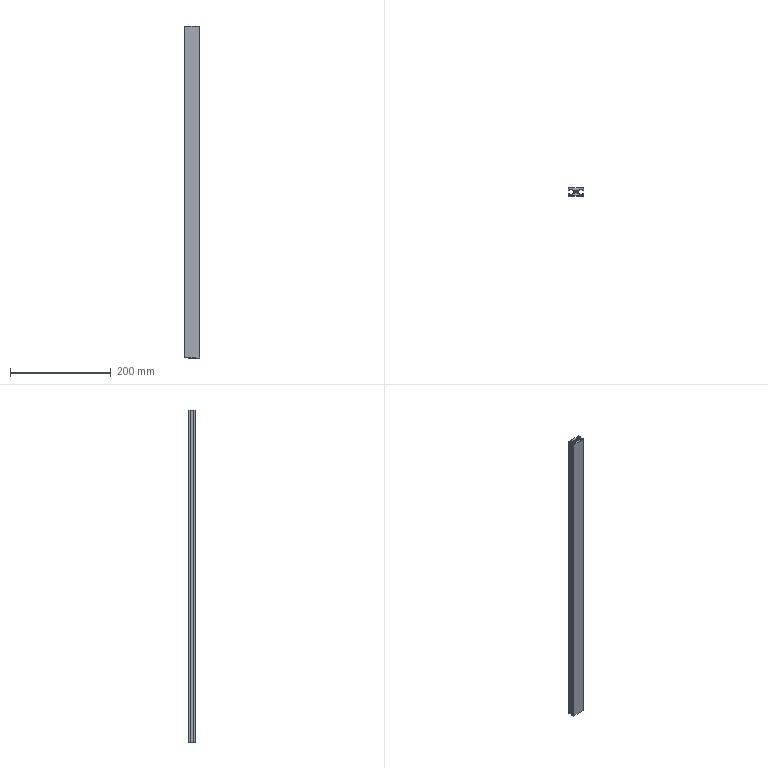Part | SolidWorks | features BaseBody 1, MoveFace 1 | 1 solid | 53 faces | box 30 x 15 x 660 mm | volume 159171 mm3 | plane 38 | cylinder 15 | commonest cylinder face diameters 1 x6 5 x5 2 x4